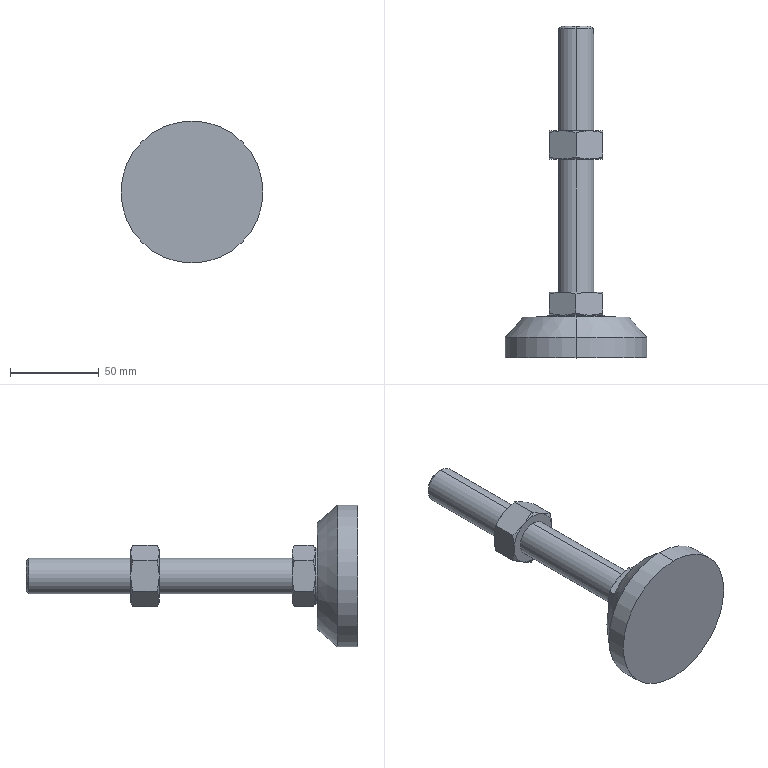Part | SolidWorks | features BaseBody 2 | 2 solids | 63 faces | box 80 x 187 x 80 mm | volume 168860 mm3 | cone 36 | plane 19 | cylinder 8 | commonest cylinder face diameters 17.294 x2 20 x2 32 x2 80 x2